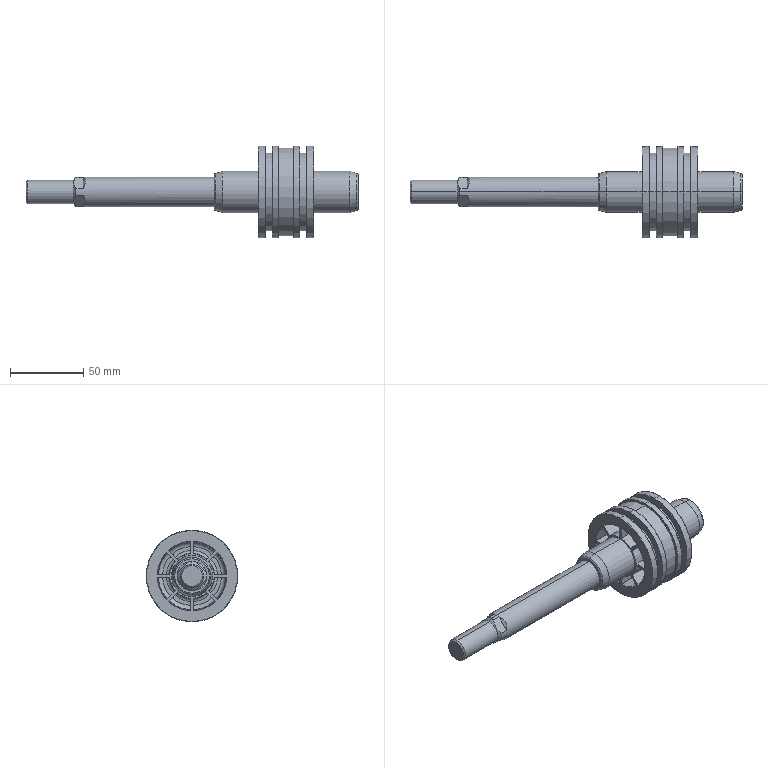Part | STEP file | 1 solid | 206 faces | box 226 x 62.5 x 62.5 mm | volume 136978 mm3 | cone 74 | plane 68 | torus 40 | cylinder 24 | commonest cylinder face diameters 62.5 x8 20 x4 28 x4 53 x4 16 x2 59.9 x2